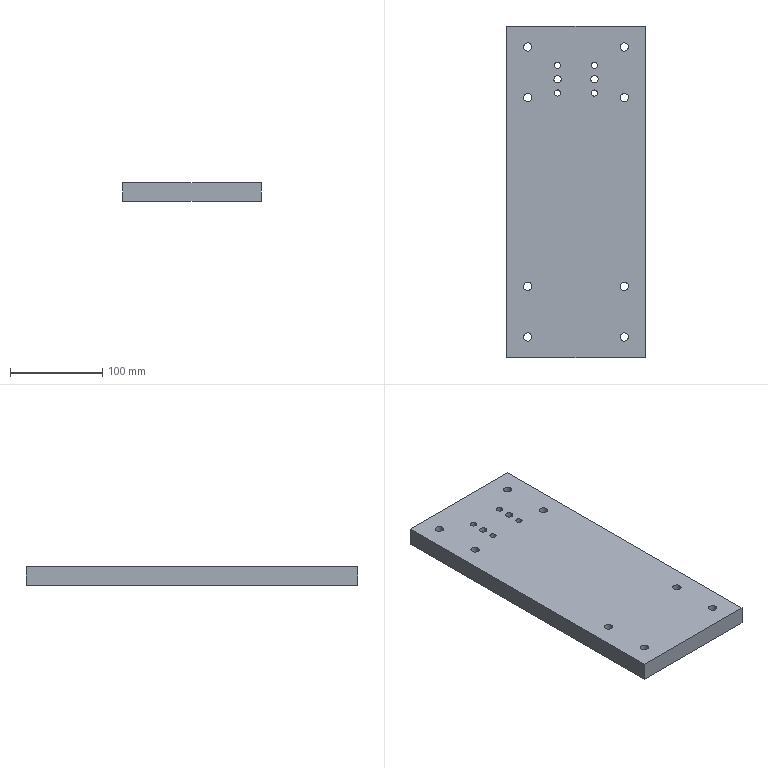Part | STEP file | SN10_010_005-04_PLACA | 1 solid | 20 faces | box 150 x 360 x 20 mm | volume 1065035 mm3 | cylinder 14 | plane 6 | commonest cylinder face diameters 9 x8 6.647 x4 8 x2